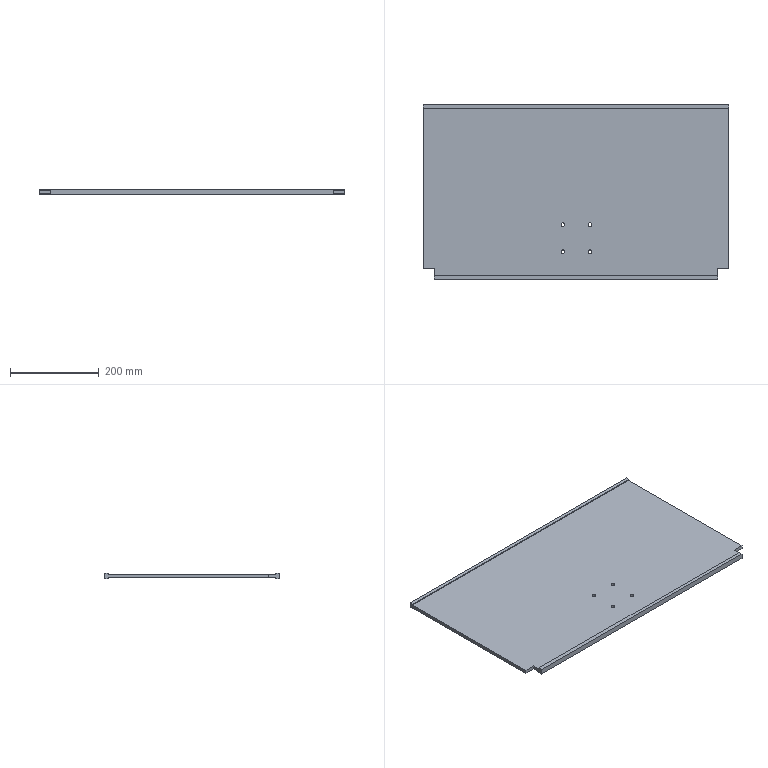Part | SolidWorks | features ICE 4, Cut 1, FlatPattern 1, SMBaseFlange 1, SheetMetal 1 | 1 solid | 26 faces | box 689 x 395 x 12 mm | volume 2213440 mm3 | plane 18 | cylinder 8 | commonest cylinder face diameters 8 x8
STEP:
#1=CARTESIAN_POINT('',(83.087,-77.137,0.));
#2=VERTEX_POINT('',#1);
#3=CARTESIAN_POINT('',(75.087,-77.137,0.));
#4=VERTEX_POINT('',#3);
#5=CARTESIAN_POINT('',(79.087,-77.137,0.));
#6=DIRECTION('',(0.,0.,-1.));
#7=DIRECTION('',(-1.,0.,0.));
#8=AXIS2_PLACEMENT_3D('',#5,#6,#7);
#9=CIRCLE('',#8,4.);
#10=EDGE_CURVE('',#2,#4,#9,.T.);
#11=ORIENTED_EDGE('',*,*,#10,.F.);
#12=CARTESIAN_POINT('',(83.087,-77.137,-8.));
#13=VERTEX_POINT('',#12);
#14=CARTESIAN_POINT('',(83.087,-77.137,2.));
#15=DIRECTION('',(0.,0.,-1.));
#16=VECTOR('',#15,1000.);
#17=LINE('',#14,#16);
#18=EDGE_CURVE('',#2,#13,#17,.T.);
#19=ORIENTED_EDGE('',*,*,#18,.T.);
#20=CARTESIAN_POINT('',(75.087,-77.137,-8.));
#21=VERTEX_POINT('',#20);
#22=CARTESIAN_POINT('',(79.087,-77.137,-8.));
#23=DIRECTION('',(0.,0.,-1.));
#24=DIRECTION('',(-1.,0.,0.));
#25=AXIS2_PLACEMENT_3D('',#22,#23,#24);
#26=CIRCLE('',#25,4.);
#27=EDGE_CURVE('',#13,#21,#26,.T.);
#28=ORIENTED_EDGE('',*,*,#27,.T.);
#29=CARTESIAN_POINT('',(75.087,-77.137,2.));
#30=DIRECTION('',(0.,0.,-1.));
#31=VECTOR('',#30,1000.);
#32=LINE('',#29,#31);
#33=EDGE_CURVE('',#4,#21,#32,.T.);
#34=ORIENTED_EDGE('',*,*,#33,.F.);
#35=EDGE_LOOP('',(#11,#19,#28,#34));
#36=FACE_OUTER_BOUND('',#35,.T.);
#37=CARTESIAN_POINT('',(79.087,-77.137,2.));
#38=DIRECTION('',(0.,0.,-1.));
#39=DIRECTION('',(-1.,0.,0.));
#40=AXIS2_PLACEMENT_3D('',#37,#38,#39);
#41=CYLINDRICAL_SURFACE('',#40,4.);
#42=ADVANCED_FACE('',(#36),#41,.F.);
#43=CARTESIAN_POINT('',(22.087,-138.137,0.));
#44=VERTEX_POINT('',#43);
#45=CARTESIAN_POINT('',(14.087,-138.137,0.));
#46=VERTEX_POINT('',#45);
#47=CARTESIAN_POINT('',(18.087,-138.137,0.));
#48=DIRECTION('',(0.,0.,-1.));
#49=DIRECTION('',(-1.,0.,0.));
#50=AXIS2_PLACEMENT_3D('',#47,#48,#49);
#51=CIRCLE('',#50,4.);
#52=EDGE_CURVE('',#44,#46,#51,.T.);
#53=ORIENTED_EDGE('',*,*,#52,.F.);
#54=CARTESIAN_POINT('',(22.087,-138.137,-8.));
#55=VERTEX_POINT('',#54);
#56=CARTESIAN_POINT('',(22.087,-138.137,2.));
#57=DIRECTION('',(0.,0.,-1.));
#58=VECTOR('',#57,1000.);
#59=LINE('',#56,#58);
#60=EDGE_CURVE('',#44,#55,#59,.T.);
#61=ORIENTED_EDGE('',*,*,#60,.T.);
#62=CARTESIAN_POINT('',(14.087,-138.137,-8.));
#63=VERTEX_POINT('',#62);
#64=CARTESIAN_POINT('',(18.087,-138.137,-8.));
#65=DIRECTION('',(0.,0.,-1.));
#66=DIRECTION('',(-1.,0.,0.));
#67=AXIS2_PLACEMENT_3D('',#64,#65,#66);
#68=CIRCLE('',#67,4.);
#69=EDGE_CURVE('',#55,#63,#68,.T.);
#70=ORIENTED_EDGE('',*,*,#69,.T.);
#71=CARTESIAN_POINT('',(14.087,-138.137,2.));
#72=DIRECTION('',(0.,0.,-1.));
#73=VECTOR('',#72,1000.);
#74=LINE('',#71,#73);
#75=EDGE_CURVE('',#46,#63,#74,.T.);
#76=ORIENTED_EDGE('',*,*,#75,.F.);
#77=EDGE_LOOP('',(#53,#61,#70,#76));
#78=FACE_OUTER_BOUND('',#77,.T.);
#79=CARTESIAN_POINT('',(18.087,-138.137,2.));
#80=DIRECTION('',(0.,0.,-1.));
#81=DIRECTION('',(-1.,0.,0.));
#82=AXIS2_PLACEMENT_3D('',#79,#80,#81);
#83=CYLINDRICAL_SURFACE('',#82,4.);
#84=ADVANCED_FACE('',(#78),#83,.F.);
#85=CARTESIAN_POINT('',(83.087,-138.137,0.));
#86=VERTEX_POINT('',#85);
#87=CARTESIAN_POINT('',(75.087,-138.137,0.));
#88=VERTEX_POINT('',#87);
#89=CARTESIAN_POINT('',(79.087,-138.137,0.));
#90=DIRECTION('',(0.,0.,-1.));
#91=DIRECTION('',(-1.,0.,0.));
#92=AXIS2_PLACEMENT_3D('',#89,#90,#91);
#93=CIRCLE('',#92,4.);
#94=EDGE_CURVE('',#86,#88,#93,.T.);
#95=ORIENTED_EDGE('',*,*,#94,.F.);
#96=CARTESIAN_POINT('',(83.087,-138.137,-8.));
#97=VERTEX_POINT('',#96);
#98=CARTESIAN_POINT('',(83.087,-138.137,2.));
#99=DIRECTION('',(0.,0.,-1.));
#100=VECTOR('',#99,1000.);
#101=LINE('',#98,#100);
#102=EDGE_CURVE('',#86,#97,#101,.T.);
#103=ORIENTED_EDGE('',*,*,#102,.T.);
#104=CARTESIAN_POINT('',(75.087,-138.137,-8.));
#105=VERTEX_POINT('',#104);
#106=CARTESIAN_POINT('',(79.087,-138.137,-8.));
#107=DIRECTION('',(0.,0.,-1.));
#108=DIRECTION('',(-1.,0.,0.));
#109=AXIS2_PLACEMENT_3D('',#106,#107,#108);
#110=CIRCLE('',#109,4.);
#111=EDGE_CURVE('',#97,#105,#110,.T.);
#112=ORIENTED_EDGE('',*,*,#111,.T.);
#113=CARTESIAN_POINT('',(75.087,-138.137,2.));
#114=DIRECTION('',(0.,0.,-1.));
#115=VECTOR('',#114,1000.);
#116=LINE('',#113,#115);
#117=EDGE_CURVE('',#88,#105,#116,.T.);
#118=ORIENTED_EDGE('',*,*,#117,.F.);
#119=EDGE_LOOP('',(#95,#103,#112,#118));
#120=FACE_OUTER_BOUND('',#119,.T.);
#121=CARTESIAN_POINT('',(79.087,-138.137,2.));
#122=DIRECTION('',(0.,0.,-1.));
#123=DIRECTION('',(-1.,0.,0.));
#124=AXIS2_PLACEMENT_3D('',#121,#122,#123);
#125=CYLINDRICAL_SURFACE('',#124,4.);
#126=ADVANCED_FACE('',(#120),#125,.F.);
#127=CARTESIAN_POINT('',(22.087,-77.137,0.));
#128=VERTEX_POINT('',#127);
#129=CARTESIAN_POINT('',(14.087,-77.137,0.));
#130=VERTEX_POINT('',#129);
#131=CARTESIAN_POINT('',(18.087,-77.137,0.));
#132=DIRECTION('',(0.,0.,-1.));
#133=DIRECTION('',(-1.,0.,0.));
#134=AXIS2_PLACEMENT_3D('',#131,#132,#133);
#135=CIRCLE('',#134,4.);
#136=EDGE_CURVE('',#128,#130,#135,.T.);
#137=ORIENTED_EDGE('',*,*,#136,.F.);
#138=CARTESIAN_POINT('',(22.087,-77.137,-8.));
#139=VERTEX_POINT('',#138);
#140=CARTESIAN_POINT('',(22.087,-77.137,2.));
#141=DIRECTION('',(0.,0.,-1.));
#142=VECTOR('',#141,1000.);
#143=LINE('',#140,#142);
#144=EDGE_CURVE('',#128,#139,#143,.T.);
#145=ORIENTED_EDGE('',*,*,#144,.T.);
#146=CARTESIAN_POINT('',(14.087,-77.137,-8.));
#147=VERTEX_POINT('',#146);
#148=CARTESIAN_POINT('',(18.087,-77.137,-8.));
#149=DIRECTION('',(0.,0.,-1.));
#150=DIRECTION('',(-1.,0.,0.));
#151=AXIS2_PLACEMENT_3D('',#148,#149,#150);
#152=CIRCLE('',#151,4.);
#153=EDGE_CURVE('',#139,#147,#152,.T.);
#154=ORIENTED_EDGE('',*,*,#153,.T.);
#155=CARTESIAN_POINT('',(14.087,-77.137,2.));
#156=DIRECTION('',(0.,0.,-1.));
#157=VECTOR('',#156,1000.);
#158=LINE('',#155,#157);
#159=EDGE_CURVE('',#130,#147,#158,.T.);
#160=ORIENTED_EDGE('',*,*,#159,.F.);
#161=EDGE_LOOP('',(#137,#145,#154,#160));
#162=FACE_OUTER_BOUND('',#161,.T.);
#163=CARTESIAN_POINT('',(18.087,-77.137,2.));
#164=DIRECTION('',(0.,0.,-1.));
#165=DIRECTION('',(-1.,0.,0.));
#166=AXIS2_PLACEMENT_3D('',#163,#164,#165);
#167=CYLINDRICAL_SURFACE('',#166,4.);
#168=ADVANCED_FACE('',(#162),#167,.F.);
#169=CARTESIAN_POINT('',(-297.,194.,-10.));
#170=VERTEX_POINT('',#169);
#171=CARTESIAN_POINT('',(-297.,194.,2.));
#172=VERTEX_POINT('',#171);
#173=CARTESIAN_POINT('',(-297.,194.,-8.));
#174=DIRECTION('',(0.,0.,1.));
#175=VECTOR('',#174,1000.);
#176=LINE('',#173,#175);
#177=EDGE_CURVE('',#170,#172,#176,.T.);
#178=ORIENTED_EDGE('',*,*,#177,.T.);
#179=CARTESIAN_POINT('',(392.,194.,2.));
#180=VERTEX_POINT('',#179);
#181=CARTESIAN_POINT('',(378.,194.,2.));
#182=DIRECTION('',(-1.,0.,0.));
#183=VECTOR('',#182,1000.);
#184=LINE('',#181,#183);
#185=EDGE_CURVE('',#180,#172,#184,.T.);
#186=ORIENTED_EDGE('',*,*,#185,.F.);
#187=CARTESIAN_POINT('',(392.,194.,-10.));
#188=VERTEX_POINT('',#187);
#189=CARTESIAN_POINT('',(392.,194.,-10.));
#190=DIRECTION('',(0.,0.,1.));
#191=VECTOR('',#190,1000.);
#192=LINE('',#189,#191);
#193=EDGE_CURVE('',#188,#180,#192,.T.);
#194=ORIENTED_EDGE('',*,*,#193,.F.);
#195=CARTESIAN_POINT('',(378.,194.,-10.));
#196=DIRECTION('',(-1.,0.,0.));
#197=VECTOR('',#196,1000.);
#198=LINE('',#195,#197);
#199=EDGE_CURVE('',#188,#170,#198,.T.);
#200=ORIENTED_EDGE('',*,*,#199,.T.);
#201=EDGE_LOOP('',(#178,#186,#194,#200));
#202=FACE_OUTER_BOUND('',#201,.T.);
#203=CARTESIAN_POINT('',(-297.,194.,-8.));
#204=DIRECTION('',(0.,1.,0.));
#205=DIRECTION('',(0.,0.,1.));
#206=AXIS2_PLACEMENT_3D('',#203,#204,#205);
#207=PLANE('',#206);
#208=ADVANCED_FACE('',(#202),#207,.T.);
#209=CARTESIAN_POINT('',(367.,-201.,-10.));
#210=VERTEX_POINT('',#209);
#211=CARTESIAN_POINT('',(367.,-201.,2.));
#212=VERTEX_POINT('',#211);
#213=CARTESIAN_POINT('',(367.,-201.,-10.));
#214=DIRECTION('',(0.,0.,1.));
#215=VECTOR('',#214,1000.);
#216=LINE('',#213,#215);
#217=EDGE_CURVE('',#210,#212,#216,.T.);
#218=ORIENTED_EDGE('',*,*,#217,.T.);
#219=CARTESIAN_POINT('',(-272.,-201.,2.));
#220=VERTEX_POINT('',#219);
#221=CARTESIAN_POINT('',(378.,-201.,2.));
#222=DIRECTION('',(-1.,0.,0.));
#223=VECTOR('',#222,1000.);
#224=LINE('',#221,#223);
#225=EDGE_CURVE('',#212,#220,#224,.T.);
#226=ORIENTED_EDGE('',*,*,#225,.T.);
#227=CARTESIAN_POINT('',(-272.,-201.,-10.));
#228=VERTEX_POINT('',#227);
#229=CARTESIAN_POINT('',(-272.,-201.,-10.));
#230=DIRECTION('',(0.,0.,1.));
#231=VECTOR('',#230,1000.);
#232=LINE('',#229,#231);
#233=EDGE_CURVE('',#228,#220,#232,.T.);
#234=ORIENTED_EDGE('',*,*,#233,.F.);
#235=CARTESIAN_POINT('',(378.,-201.,-10.));
#236=DIRECTION('',(-1.,0.,0.));
#237=VECTOR('',#236,1000.);
#238=LINE('',#235,#237);
#239=EDGE_CURVE('',#210,#228,#238,.T.);
#240=ORIENTED_EDGE('',*,*,#239,.F.);
#241=EDGE_LOOP('',(#218,#226,#234,#240));
#242=FACE_OUTER_BOUND('',#241,.T.);
#243=CARTESIAN_POINT('',(-297.,-201.,-8.));
#244=DIRECTION('',(0.,-1.,0.));
#245=DIRECTION('',(0.,0.,-1.));
#246=AXIS2_PLACEMENT_3D('',#243,#244,#245);
#247=PLANE('',#246);
#248=ADVANCED_FACE('',(#242),#247,.T.);
#249=CARTESIAN_POINT('',(-297.,-176.,-8.));
#250=VERTEX_POINT('',#249);
#251=CARTESIAN_POINT('',(-297.,-176.,0.));
#252=VERTEX_POINT('',#251);
#253=CARTESIAN_POINT('',(-297.,-176.,-10.));
#254=DIRECTION('',(0.,0.,1.));
#255=VECTOR('',#254,1000.);
#256=LINE('',#253,#255);
#257=EDGE_CURVE('',#250,#252,#256,.T.);
#258=ORIENTED_EDGE('',*,*,#257,.T.);
#259=CARTESIAN_POINT('',(-297.,185.,0.));
#260=VERTEX_POINT('',#259);
#261=CARTESIAN_POINT('',(-297.,194.,0.));
#262=DIRECTION('',(0.,-1.,0.));
#263=VECTOR('',#262,1000.);
#264=LINE('',#261,#263);
#265=EDGE_CURVE('',#260,#252,#264,.T.);
#266=ORIENTED_EDGE('',*,*,#265,.F.);
#267=CARTESIAN_POINT('',(-297.,185.,2.));
#268=VERTEX_POINT('',#267);
#269=CARTESIAN_POINT('',(-297.,185.,-10.));
#270=DIRECTION('',(0.,0.,1.));
#271=VECTOR('',#270,1000.);
#272=LINE('',#269,#271);
#273=EDGE_CURVE('',#260,#268,#272,.T.);
#274=ORIENTED_EDGE('',*,*,#273,.T.);
#275=CARTESIAN_POINT('',(-297.,194.,2.));
#276=DIRECTION('',(0.,1.,0.));
#277=VECTOR('',#276,1000.);
#278=LINE('',#275,#277);
#279=EDGE_CURVE('',#268,#172,#278,.T.);
#280=ORIENTED_EDGE('',*,*,#279,.T.);
#281=ORIENTED_EDGE('',*,*,#177,.F.);
#282=CARTESIAN_POINT('',(-297.,185.,-10.));
#283=VERTEX_POINT('',#282);
#284=CARTESIAN_POINT('',(-297.,194.,-10.));
#285=DIRECTION('',(0.,-1.,0.));
#286=VECTOR('',#285,1000.);
#287=LINE('',#284,#286);
#288=EDGE_CURVE('',#170,#283,#287,.T.);
#289=ORIENTED_EDGE('',*,*,#288,.T.);
#290=CARTESIAN_POINT('',(-297.,185.,-8.));
#291=VERTEX_POINT('',#290);
#292=CARTESIAN_POINT('',(-297.,185.,-10.));
#293=DIRECTION('',(0.,0.,1.));
#294=VECTOR('',#293,1000.);
#295=LINE('',#292,#294);
#296=EDGE_CURVE('',#283,#291,#295,.T.);
#297=ORIENTED_EDGE('',*,*,#296,.T.);
#298=CARTESIAN_POINT('',(-297.,194.,-8.));
#299=DIRECTION('',(0.,-1.,0.));
#300=VECTOR('',#299,1000.);
#301=LINE('',#298,#300);
#302=EDGE_CURVE('',#291,#250,#301,.T.);
#303=ORIENTED_EDGE('',*,*,#302,.T.);
#304=EDGE_LOOP('',(#258,#266,#274,#280,#281,#289,#297,#303));
#305=FACE_OUTER_BOUND('',#304,.T.);
#306=CARTESIAN_POINT('',(-297.,194.,-8.));
#307=DIRECTION('',(-1.,0.,0.));
#308=DIRECTION('',(0.,0.,1.));
#309=AXIS2_PLACEMENT_3D('',#306,#307,#308);
#310=PLANE('',#309);
#311=ADVANCED_FACE('',(#305),#310,.T.);
#312=CARTESIAN_POINT('',(367.,-192.,-8.));
#313=VERTEX_POINT('',#312);
#314=CARTESIAN_POINT('',(367.,-176.,-8.));
#315=VERTEX_POINT('',#314);
#316=CARTESIAN_POINT('',(367.,0.,-8.));
#317=DIRECTION('',(0.,1.,0.));
#318=VECTOR('',#317,1000.);
#319=LINE('',#316,#318);
#320=EDGE_CURVE('',#313,#315,#319,.T.);
#321=ORIENTED_EDGE('',*,*,#320,.F.);
#322=CARTESIAN_POINT('',(-272.,-192.,-8.));
#323=VERTEX_POINT('',#322);
#324=CARTESIAN_POINT('',(0.,-192.,-8.));
#325=DIRECTION('',(1.,0.,0.));
#326=VECTOR('',#325,1000.);
#327=LINE('',#324,#326);
#328=EDGE_CURVE('',#323,#313,#327,.T.);
#329=ORIENTED_EDGE('',*,*,#328,.F.);
#330=CARTESIAN_POINT('',(-272.,-176.,-8.));
#331=VERTEX_POINT('',#330);
#332=CARTESIAN_POINT('',(-272.,0.,-8.));
#333=DIRECTION('',(0.,-1.,0.));
#334=VECTOR('',#333,1000.);
#335=LINE('',#332,#334);
#336=EDGE_CURVE('',#331,#323,#335,.T.);
#337=ORIENTED_EDGE('',*,*,#336,.F.);
#338=CARTESIAN_POINT('',(0.,-176.,-8.));
#339=DIRECTION('',(1.,0.,0.));
#340=VECTOR('',#339,1000.);
#341=LINE('',#338,#340);
#342=EDGE_CURVE('',#250,#331,#341,.T.);
#343=ORIENTED_EDGE('',*,*,#342,.F.);
#344=ORIENTED_EDGE('',*,*,#302,.F.);
#345=CARTESIAN_POINT('',(392.,185.,-8.));
#346=VERTEX_POINT('',#345);
#347=CARTESIAN_POINT('',(0.,185.,-8.));
#348=DIRECTION('',(-1.,0.,0.));
#349=VECTOR('',#348,1000.);
#350=LINE('',#347,#349);
#351=EDGE_CURVE('',#346,#291,#350,.T.);
#352=ORIENTED_EDGE('',*,*,#351,.F.);
#353=CARTESIAN_POINT('',(392.,-176.,-8.));
#354=VERTEX_POINT('',#353);
#355=CARTESIAN_POINT('',(392.,-192.,-8.));
#356=DIRECTION('',(0.,1.,0.));
#357=VECTOR('',#356,1000.);
#358=LINE('',#355,#357);
#359=EDGE_CURVE('',#354,#346,#358,.T.);
#360=ORIENTED_EDGE('',*,*,#359,.F.);
#361=CARTESIAN_POINT('',(0.,-176.,-8.));
#362=DIRECTION('',(1.,0.,0.));
#363=VECTOR('',#362,1000.);
#364=LINE('',#361,#363);
#365=EDGE_CURVE('',#315,#354,#364,.T.);
#366=ORIENTED_EDGE('',*,*,#365,.F.);
#367=EDGE_LOOP('',(#321,#329,#337,#343,#344,#352,#360,#366));
#368=FACE_OUTER_BOUND('',#367,.T.);
#369=CARTESIAN_POINT('',(79.087,-77.137,-8.));
#370=DIRECTION('',(0.,0.,-1.));
#371=DIRECTION('',(-1.,0.,0.));
#372=AXIS2_PLACEMENT_3D('',#369,#370,#371);
#373=CIRCLE('',#372,4.);
#374=EDGE_CURVE('',#21,#13,#373,.T.);
#375=ORIENTED_EDGE('',*,*,#374,.F.);
#376=ORIENTED_EDGE('',*,*,#27,.F.);
#377=EDGE_LOOP('',(#375,#376));
#378=FACE_BOUND('',#377,.T.);
#379=CARTESIAN_POINT('',(18.087,-138.137,-8.));
#380=DIRECTION('',(0.,0.,-1.));
#381=DIRECTION('',(-1.,0.,0.));
#382=AXIS2_PLACEMENT_3D('',#379,#380,#381);
#383=CIRCLE('',#382,4.);
#384=EDGE_CURVE('',#63,#55,#383,.T.);
#385=ORIENTED_EDGE('',*,*,#384,.F.);
#386=ORIENTED_EDGE('',*,*,#69,.F.);
#387=EDGE_LOOP('',(#385,#386));
#388=FACE_BOUND('',#387,.T.);
#389=CARTESIAN_POINT('',(79.087,-138.137,-8.));
#390=DIRECTION('',(0.,0.,-1.));
#391=DIRECTION('',(-1.,0.,0.));
#392=AXIS2_PLACEMENT_3D('',#389,#390,#391);
#393=CIRCLE('',#392,4.);
#394=EDGE_CURVE('',#105,#97,#393,.T.);
#395=ORIENTED_EDGE('',*,*,#394,.F.);
#396=ORIENTED_EDGE('',*,*,#111,.F.);
#397=EDGE_LOOP('',(#395,#396));
#398=FACE_BOUND('',#397,.T.);
#399=CARTESIAN_POINT('',(18.087,-77.137,-8.));
#400=DIRECTION('',(0.,0.,-1.));
#401=DIRECTION('',(-1.,0.,0.));
#402=AXIS2_PLACEMENT_3D('',#399,#400,#401);
#403=CIRCLE('',#402,4.);
#404=EDGE_CURVE('',#147,#139,#403,.T.);
#405=ORIENTED_EDGE('',*,*,#404,.F.);
#406=ORIENTED_EDGE('',*,*,#153,.F.);
#407=EDGE_LOOP('',(#405,#406));
#408=FACE_BOUND('',#407,.T.);
#409=CARTESIAN_POINT('',(0.,0.,-8.));
#410=DIRECTION('',(0.,0.,-1.));
#411=DIRECTION('',(-1.,0.,0.));
#412=AXIS2_PLACEMENT_3D('',#409,#410,#411);
#413=PLANE('',#412);
#414=ADVANCED_FACE('',(#368,#378,#388,#398,#408),#413,.T.);
#415=CARTESIAN_POINT('',(79.087,-77.137,0.));
#416=DIRECTION('',(0.,0.,-1.));
#417=DIRECTION('',(-1.,0.,0.));
#418=AXIS2_PLACEMENT_3D('',#415,#416,#417);
#419=CIRCLE('',#418,4.);
#420=EDGE_CURVE('',#4,#2,#419,.T.);
#421=ORIENTED_EDGE('',*,*,#420,.T.);
#422=ORIENTED_EDGE('',*,*,#10,.T.);
#423=EDGE_LOOP('',(#421,#422));
#424=FACE_BOUND('',#423,.T.);
#425=CARTESIAN_POINT('',(18.087,-138.137,0.));
#426=DIRECTION('',(0.,0.,-1.));
#427=DIRECTION('',(-1.,0.,0.));
#428=AXIS2_PLACEMENT_3D('',#425,#426,#427);
#429=CIRCLE('',#428,4.);
#430=EDGE_CURVE('',#46,#44,#429,.T.);
#431=ORIENTED_EDGE('',*,*,#430,.T.);
#432=ORIENTED_EDGE('',*,*,#52,.T.);
#433=EDGE_LOOP('',(#431,#432));
#434=FACE_BOUND('',#433,.T.);
#435=CARTESIAN_POINT('',(79.087,-138.137,0.));
#436=DIRECTION('',(0.,0.,-1.));
#437=DIRECTION('',(-1.,0.,0.));
#438=AXIS2_PLACEMENT_3D('',#435,#436,#437);
#439=CIRCLE('',#438,4.);
#440=EDGE_CURVE('',#88,#86,#439,.T.);
#441=ORIENTED_EDGE('',*,*,#440,.T.);
#442=ORIENTED_EDGE('',*,*,#94,.T.);
#443=EDGE_LOOP('',(#441,#442));
#444=FACE_BOUND('',#443,.T.);
#445=CARTESIAN_POINT('',(18.087,-77.137,0.));
#446=DIRECTION('',(0.,0.,-1.));
#447=DIRECTION('',(-1.,0.,0.));
#448=AXIS2_PLACEMENT_3D('',#445,#446,#447);
#449=CIRCLE('',#448,4.);
#450=EDGE_CURVE('',#130,#128,#449,.T.);
#451=ORIENTED_EDGE('',*,*,#450,.T.);
#452=ORIENTED_EDGE('',*,*,#136,.T.);
#453=EDGE_LOOP('',(#451,#452));
#454=FACE_BOUND('',#453,.T.);
#455=CARTESIAN_POINT('',(-272.,-192.,0.));
#456=VERTEX_POINT('',#455);
#457=CARTESIAN_POINT('',(367.,-192.,0.));
#458=VERTEX_POINT('',#457);
#459=CARTESIAN_POINT('',(0.,-192.,0.));
#460=DIRECTION('',(1.,0.,0.));
#461=VECTOR('',#460,1000.);
#462=LINE('',#459,#461);
#463=EDGE_CURVE('',#456,#458,#462,.T.);
#464=ORIENTED_EDGE('',*,*,#463,.T.);
#465=CARTESIAN_POINT('',(367.,-176.,0.));
#466=VERTEX_POINT('',#465);
#467=CARTESIAN_POINT('',(367.,0.,0.));
#468=DIRECTION('',(0.,1.,0.));
#469=VECTOR('',#468,1000.);
#470=LINE('',#467,#469);
#471=EDGE_CURVE('',#458,#466,#470,.T.);
#472=ORIENTED_EDGE('',*,*,#471,.T.);
#473=CARTESIAN_POINT('',(392.,-176.,0.));
#474=VERTEX_POINT('',#473);
#475=CARTESIAN_POINT('',(0.,-176.,0.));
#476=DIRECTION('',(1.,0.,0.));
#477=VECTOR('',#476,1000.);
#478=LINE('',#475,#477);
#479=EDGE_CURVE('',#466,#474,#478,.T.);
#480=ORIENTED_EDGE('',*,*,#479,.T.);
#481=CARTESIAN_POINT('',(392.,185.,0.));
#482=VERTEX_POINT('',#481);
#483=CARTESIAN_POINT('',(392.,185.,0.));
#484=DIRECTION('',(0.,-1.,0.));
#485=VECTOR('',#484,1000.);
#486=LINE('',#483,#485);
#487=EDGE_CURVE('',#482,#474,#486,.T.);
#488=ORIENTED_EDGE('',*,*,#487,.F.);
#489=CARTESIAN_POINT('',(0.,185.,0.));
#490=DIRECTION('',(-1.,0.,0.));
#491=VECTOR('',#490,1000.);
#492=LINE('',#489,#491);
#493=EDGE_CURVE('',#482,#260,#492,.T.);
#494=ORIENTED_EDGE('',*,*,#493,.T.);
#495=ORIENTED_EDGE('',*,*,#265,.T.);
#496=CARTESIAN_POINT('',(-272.,-176.,0.));
#497=VERTEX_POINT('',#496);
#498=CARTESIAN_POINT('',(0.,-176.,0.));
#499=DIRECTION('',(1.,0.,0.));
#500=VECTOR('',#499,1000.);
#501=LINE('',#498,#500);
#502=EDGE_CURVE('',#252,#497,#501,.T.);
#503=ORIENTED_EDGE('',*,*,#502,.T.);
#504=CARTESIAN_POINT('',(-272.,0.,0.));
#505=DIRECTION('',(0.,-1.,0.));
#506=VECTOR('',#505,1000.);
#507=LINE('',#504,#506);
#508=EDGE_CURVE('',#497,#456,#507,.T.);
#509=ORIENTED_EDGE('',*,*,#508,.T.);
#510=EDGE_LOOP('',(#464,#472,#480,#488,#494,#495,#503,#509));
#511=FACE_OUTER_BOUND('',#510,.T.);
#512=CARTESIAN_POINT('',(0.,0.,0.));
#513=DIRECTION('',(0.,0.,-1.));
#514=DIRECTION('',(-1.,0.,0.));
#515=AXIS2_PLACEMENT_3D('',#512,#513,#514);
#516=PLANE('',#515);
#517=ADVANCED_FACE('',(#424,#434,#444,#454,#511),#516,.F.);
#518=CARTESIAN_POINT('',(367.,-192.,2.));
#519=VERTEX_POINT('',#518);
#520=CARTESIAN_POINT('',(367.,-201.,2.));
#521=DIRECTION('',(0.,-1.,0.));
#522=VECTOR('',#521,1000.);
#523=LINE('',#520,#522);
#524=EDGE_CURVE('',#519,#212,#523,.T.);
#525=ORIENTED_EDGE('',*,*,#524,.F.);
#526=CARTESIAN_POINT('',(-272.,-192.,2.));
#527=VERTEX_POINT('',#526);
#528=CARTESIAN_POINT('',(378.,-192.,2.));
#529=DIRECTION('',(-1.,0.,0.));
#530=VECTOR('',#529,1000.);
#531=LINE('',#528,#530);
#532=EDGE_CURVE('',#519,#527,#531,.T.);
#533=ORIENTED_EDGE('',*,*,#532,.T.);
#534=CARTESIAN_POINT('',(-272.,-201.,2.));
#535=DIRECTION('',(0.,1.,0.));
#536=VECTOR('',#535,1000.);
#537=LINE('',#534,#536);
#538=EDGE_CURVE('',#220,#527,#537,.T.);
#539=ORIENTED_EDGE('',*,*,#538,.F.);
#540=ORIENTED_EDGE('',*,*,#225,.F.);
#541=EDGE_LOOP('',(#525,#533,#539,#540));
#542=FACE_OUTER_BOUND('',#541,.T.);
#543=CARTESIAN_POINT('',(378.,-201.,2.));
#544=DIRECTION('',(0.,0.,1.));
#545=DIRECTION('',(1.,0.,0.));
#546=AXIS2_PLACEMENT_3D('',#543,#544,#545);
#547=PLANE('',#546);
#548=ADVANCED_FACE('',(#542),#547,.T.);
#549=CARTESIAN_POINT('',(367.,-192.,-10.));
#550=DIRECTION('',(0.,0.,1.));
#551=VECTOR('',#550,1000.);
#552=LINE('',#549,#551);
#553=EDGE_CURVE('',#458,#519,#552,.T.);
#554=ORIENTED_EDGE('',*,*,#553,.F.);
#555=ORIENTED_EDGE('',*,*,#463,.F.);
#556=CARTESIAN_POINT('',(-272.,-192.,-10.));
#557=DIRECTION('',(0.,0.,-1.));
#558=VECTOR('',#557,1000.);
#559=LINE('',#556,#558);
#560=EDGE_CURVE('',#527,#456,#559,.T.);
#561=ORIENTED_EDGE('',*,*,#560,.F.);
#562=ORIENTED_EDGE('',*,*,#532,.F.);
#563=EDGE_LOOP('',(#554,#555,#561,#562));
#564=FACE_OUTER_BOUND('',#563,.T.);
#565=CARTESIAN_POINT('',(378.,-192.,-10.));
#566=DIRECTION('',(0.,1.,0.));
#567=DIRECTION('',(0.,0.,1.));
#568=AXIS2_PLACEMENT_3D('',#565,#566,#567);
#569=PLANE('',#568);
#570=ADVANCED_FACE('',(#564),#569,.T.);
#571=CARTESIAN_POINT('',(367.,-192.,-10.));
#572=VERTEX_POINT('',#571);
#573=CARTESIAN_POINT('',(367.,-192.,-10.));
#574=DIRECTION('',(0.,0.,1.));
#575=VECTOR('',#574,1000.);
#576=LINE('',#573,#575);
#577=EDGE_CURVE('',#572,#313,#576,.T.);
#578=ORIENTED_EDGE('',*,*,#577,.F.);
#579=CARTESIAN_POINT('',(-272.,-192.,-10.));
#580=VERTEX_POINT('',#579);
#581=CARTESIAN_POINT('',(378.,-192.,-10.));
#582=DIRECTION('',(-1.,0.,0.));
#583=VECTOR('',#582,1000.);
#584=LINE('',#581,#583);
#585=EDGE_CURVE('',#572,#580,#584,.T.);
#586=ORIENTED_EDGE('',*,*,#585,.T.);
#587=CARTESIAN_POINT('',(-272.,-192.,-10.));
#588=DIRECTION('',(0.,0.,-1.));
#589=VECTOR('',#588,1000.);
#590=LINE('',#587,#589);
#591=EDGE_CURVE('',#323,#580,#590,.T.);
#592=ORIENTED_EDGE('',*,*,#591,.F.);
#593=ORIENTED_EDGE('',*,*,#328,.T.);
#594=EDGE_LOOP('',(#578,#586,#592,#593));
#595=FACE_OUTER_BOUND('',#594,.T.);
#596=CARTESIAN_POINT('',(378.,-192.,-10.));
#597=DIRECTION('',(0.,1.,0.));
#598=DIRECTION('',(0.,0.,1.));
#599=AXIS2_PLACEMENT_3D('',#596,#597,#598);
#600=PLANE('',#599);
#601=ADVANCED_FACE('',(#595),#600,.T.);
#602=CARTESIAN_POINT('',(367.,-201.,-10.));
#603=DIRECTION('',(0.,-1.,0.));
#604=VECTOR('',#603,1000.);
#605=LINE('',#602,#604);
#606=EDGE_CURVE('',#572,#210,#605,.T.);
#607=ORIENTED_EDGE('',*,*,#606,.T.);
#608=ORIENTED_EDGE('',*,*,#239,.T.);
#609=CARTESIAN_POINT('',(-272.,-201.,-10.));
#610=DIRECTION('',(0.,1.,0.));
#611=VECTOR('',#610,1000.);
#612=LINE('',#609,#611);
#613=EDGE_CURVE('',#228,#580,#612,.T.);
#614=ORIENTED_EDGE('',*,*,#613,.T.);
#615=ORIENTED_EDGE('',*,*,#585,.F.);
#616=EDGE_LOOP('',(#607,#608,#614,#615));
#617=FACE_OUTER_BOUND('',#616,.T.);
#618=CARTESIAN_POINT('',(378.,-201.,-10.));
#619=DIRECTION('',(0.,0.,-1.));
#620=DIRECTION('',(-1.,0.,0.));
#621=AXIS2_PLACEMENT_3D('',#618,#619,#620);
#622=PLANE('',#621);
#623=ADVANCED_FACE('',(#617),#622,.T.);
#624=CARTESIAN_POINT('',(392.,185.,2.));
#625=VERTEX_POINT('',#624);
#626=CARTESIAN_POINT('',(378.,185.,2.));
#627=DIRECTION('',(-1.,0.,0.));
#628=VECTOR('',#627,1000.);
#629=LINE('',#626,#628);
#630=EDGE_CURVE('',#625,#268,#629,.T.);
#631=ORIENTED_EDGE('',*,*,#630,.F.);
#632=CARTESIAN_POINT('',(392.,194.,2.));
#633=DIRECTION('',(0.,-1.,0.));
#634=VECTOR('',#633,1000.);
#635=LINE('',#632,#634);
#636=EDGE_CURVE('',#180,#625,#635,.T.);
#637=ORIENTED_EDGE('',*,*,#636,.F.);
#638=ORIENTED_EDGE('',*,*,#185,.T.);
#639=ORIENTED_EDGE('',*,*,#279,.F.);
#640=EDGE_LOOP('',(#631,#637,#638,#639));
#641=FACE_OUTER_BOUND('',#640,.T.);
#642=CARTESIAN_POINT('',(378.,194.,2.));
#643=DIRECTION('',(0.,0.,1.));
#644=DIRECTION('',(1.,0.,0.));
#645=AXIS2_PLACEMENT_3D('',#642,#643,#644);
#646=PLANE('',#645);
#647=ADVANCED_FACE('',(#641),#646,.T.);
#648=ORIENTED_EDGE('',*,*,#493,.F.);
#649=CARTESIAN_POINT('',(392.,185.,2.));
#650=DIRECTION('',(0.,0.,-1.));
#651=VECTOR('',#650,1000.);
#652=LINE('',#649,#651);
#653=EDGE_CURVE('',#625,#482,#652,.T.);
#654=ORIENTED_EDGE('',*,*,#653,.F.);
#655=ORIENTED_EDGE('',*,*,#630,.T.);
#656=ORIENTED_EDGE('',*,*,#273,.F.);
#657=EDGE_LOOP('',(#648,#654,#655,#656));
#658=FACE_OUTER_BOUND('',#657,.T.);
#659=CARTESIAN_POINT('',(378.,185.,-10.));
#660=DIRECTION('',(0.,-1.,0.));
#661=DIRECTION('',(0.,0.,-1.));
#662=AXIS2_PLACEMENT_3D('',#659,#660,#661);
#663=PLANE('',#662);
#664=ADVANCED_FACE('',(#658),#663,.T.);
#665=ORIENTED_EDGE('',*,*,#199,.F.);
#666=CARTESIAN_POINT('',(392.,185.,-10.));
#667=VERTEX_POINT('',#666);
#668=CARTESIAN_POINT('',(392.,185.,-10.));
#669=DIRECTION('',(0.,1.,0.));
#670=VECTOR('',#669,1000.);
#671=LINE('',#668,#670);
#672=EDGE_CURVE('',#667,#188,#671,.T.);
#673=ORIENTED_EDGE('',*,*,#672,.F.);
#674=CARTESIAN_POINT('',(378.,185.,-10.));
#675=DIRECTION('',(-1.,0.,0.));
#676=VECTOR('',#675,1000.);
#677=LINE('',#674,#676);
#678=EDGE_CURVE('',#667,#283,#677,.T.);
#679=ORIENTED_EDGE('',*,*,#678,.T.);
#680=ORIENTED_EDGE('',*,*,#288,.F.);
#681=EDGE_LOOP('',(#665,#673,#679,#680));
#682=FACE_OUTER_BOUND('',#681,.T.);
#683=CARTESIAN_POINT('',(378.,194.,-10.));
#684=DIRECTION('',(0.,0.,-1.));
#685=DIRECTION('',(-1.,0.,0.));
#686=AXIS2_PLACEMENT_3D('',#683,#684,#685);
#687=PLANE('',#686);
#688=ADVANCED_FACE('',(#682),#687,.T.);
#689=ORIENTED_EDGE('',*,*,#678,.F.);
#690=CARTESIAN_POINT('',(392.,185.,-8.));
#691=DIRECTION('',(0.,0.,-1.));
#692=VECTOR('',#691,1000.);
#693=LINE('',#690,#692);
#694=EDGE_CURVE('',#346,#667,#693,.T.);
#695=ORIENTED_EDGE('',*,*,#694,.F.);
#696=ORIENTED_EDGE('',*,*,#351,.T.);
#697=ORIENTED_EDGE('',*,*,#296,.F.);
#698=EDGE_LOOP('',(#689,#695,#696,#697));
#699=FACE_OUTER_BOUND('',#698,.T.);
#700=CARTESIAN_POINT('',(378.,185.,-10.));
#701=DIRECTION('',(0.,-1.,0.));
#702=DIRECTION('',(0.,0.,-1.));
#703=AXIS2_PLACEMENT_3D('',#700,#701,#702);
#704=PLANE('',#703);
#705=ADVANCED_FACE('',(#699),#704,.T.);
#706=ORIENTED_EDGE('',*,*,#144,.F.);
#707=ORIENTED_EDGE('',*,*,#450,.F.);
#708=ORIENTED_EDGE('',*,*,#159,.T.);
#709=ORIENTED_EDGE('',*,*,#404,.T.);
#710=EDGE_LOOP('',(#706,#707,#708,#709));
#711=FACE_OUTER_BOUND('',#710,.T.);
#712=CARTESIAN_POINT('',(18.087,-77.137,2.));
#713=DIRECTION('',(0.,0.,-1.));
#714=DIRECTION('',(-1.,0.,0.));
#715=AXIS2_PLACEMENT_3D('',#712,#713,#714);
#716=CYLINDRICAL_SURFACE('',#715,4.);
#717=ADVANCED_FACE('',(#711),#716,.F.);
#718=ORIENTED_EDGE('',*,*,#102,.F.);
#719=ORIENTED_EDGE('',*,*,#440,.F.);
#720=ORIENTED_EDGE('',*,*,#117,.T.);
#721=ORIENTED_EDGE('',*,*,#394,.T.);
#722=EDGE_LOOP('',(#718,#719,#720,#721));
#723=FACE_OUTER_BOUND('',#722,.T.);
#724=CARTESIAN_POINT('',(79.087,-138.137,2.));
#725=DIRECTION('',(0.,0.,-1.));
#726=DIRECTION('',(-1.,0.,0.));
#727=AXIS2_PLACEMENT_3D('',#724,#725,#726);
#728=CYLINDRICAL_SURFACE('',#727,4.);
#729=ADVANCED_FACE('',(#723),#728,.F.);
#730=ORIENTED_EDGE('',*,*,#60,.F.);
#731=ORIENTED_EDGE('',*,*,#430,.F.);
#732=ORIENTED_EDGE('',*,*,#75,.T.);
#733=ORIENTED_EDGE('',*,*,#384,.T.);
#734=EDGE_LOOP('',(#730,#731,#732,#733));
#735=FACE_OUTER_BOUND('',#734,.T.);
#736=CARTESIAN_POINT('',(18.087,-138.137,2.));
#737=DIRECTION('',(0.,0.,-1.));
#738=DIRECTION('',(-1.,0.,0.));
#739=AXIS2_PLACEMENT_3D('',#736,#737,#738);
#740=CYLINDRICAL_SURFACE('',#739,4.);
#741=ADVANCED_FACE('',(#735),#740,.F.);
#742=ORIENTED_EDGE('',*,*,#18,.F.);
#743=ORIENTED_EDGE('',*,*,#420,.F.);
#744=ORIENTED_EDGE('',*,*,#33,.T.);
#745=ORIENTED_EDGE('',*,*,#374,.T.);
#746=EDGE_LOOP('',(#742,#743,#744,#745));
#747=FACE_OUTER_BOUND('',#746,.T.);
#748=CARTESIAN_POINT('',(79.087,-77.137,2.));
#749=DIRECTION('',(0.,0.,-1.));
#750=DIRECTION('',(-1.,0.,0.));
#751=AXIS2_PLACEMENT_3D('',#748,#749,#750);
#752=CYLINDRICAL_SURFACE('',#751,4.);
#753=ADVANCED_FACE('',(#747),#752,.F.);
#754=ORIENTED_EDGE('',*,*,#342,.T.);
#755=CARTESIAN_POINT('',(-272.,-176.,-10.));
#756=DIRECTION('',(0.,0.,1.));
#757=VECTOR('',#756,1000.);
#758=LINE('',#755,#757);
#759=EDGE_CURVE('',#331,#497,#758,.T.);
#760=ORIENTED_EDGE('',*,*,#759,.T.);
#761=ORIENTED_EDGE('',*,*,#502,.F.);
#762=ORIENTED_EDGE('',*,*,#257,.F.);
#763=EDGE_LOOP('',(#754,#760,#761,#762));
#764=FACE_OUTER_BOUND('',#763,.T.);
#765=CARTESIAN_POINT('',(-297.,-176.,-10.));
#766=DIRECTION('',(0.,1.,0.));
#767=DIRECTION('',(0.,0.,1.));
#768=AXIS2_PLACEMENT_3D('',#765,#766,#767);
#769=PLANE('',#768);
#770=ADVANCED_FACE('',(#764),#769,.F.);
#771=ORIENTED_EDGE('',*,*,#759,.F.);
#772=ORIENTED_EDGE('',*,*,#336,.T.);
#773=ORIENTED_EDGE('',*,*,#591,.T.);
#774=ORIENTED_EDGE('',*,*,#613,.F.);
#775=ORIENTED_EDGE('',*,*,#233,.T.);
#776=ORIENTED_EDGE('',*,*,#538,.T.);
#777=ORIENTED_EDGE('',*,*,#560,.T.);
#778=ORIENTED_EDGE('',*,*,#508,.F.);
#779=EDGE_LOOP('',(#771,#772,#773,#774,#775,#776,#777,#778));
#780=FACE_OUTER_BOUND('',#779,.T.);
#781=CARTESIAN_POINT('',(-272.,-201.,-10.));
#782=DIRECTION('',(1.,0.,0.));
#783=DIRECTION('',(0.,0.,-1.));
#784=AXIS2_PLACEMENT_3D('',#781,#782,#783);
#785=PLANE('',#784);
#786=ADVANCED_FACE('',(#780),#785,.F.);
#787=ORIENTED_EDGE('',*,*,#487,.T.);
#788=CARTESIAN_POINT('',(392.,-176.,0.));
#789=DIRECTION('',(0.,0.,-1.));
#790=VECTOR('',#789,1000.);
#791=LINE('',#788,#790);
#792=EDGE_CURVE('',#474,#354,#791,.T.);
#793=ORIENTED_EDGE('',*,*,#792,.T.);
#794=ORIENTED_EDGE('',*,*,#359,.T.);
#795=ORIENTED_EDGE('',*,*,#694,.T.);
#796=ORIENTED_EDGE('',*,*,#672,.T.);
#797=ORIENTED_EDGE('',*,*,#193,.T.);
#798=ORIENTED_EDGE('',*,*,#636,.T.);
#799=ORIENTED_EDGE('',*,*,#653,.T.);
#800=EDGE_LOOP('',(#787,#793,#794,#795,#796,#797,#798,#799));
#801=FACE_OUTER_BOUND('',#800,.T.);
#802=CARTESIAN_POINT('',(392.,0.,0.));
#803=DIRECTION('',(-1.,0.,0.));
#804=DIRECTION('',(0.,0.,1.));
#805=AXIS2_PLACEMENT_3D('',#802,#803,#804);
#806=PLANE('',#805);
#807=ADVANCED_FACE('',(#801),#806,.F.);
#808=ORIENTED_EDGE('',*,*,#553,.T.);
#809=ORIENTED_EDGE('',*,*,#524,.T.);
#810=ORIENTED_EDGE('',*,*,#217,.F.);
#811=ORIENTED_EDGE('',*,*,#606,.F.);
#812=ORIENTED_EDGE('',*,*,#577,.T.);
#813=ORIENTED_EDGE('',*,*,#320,.T.);
#814=CARTESIAN_POINT('',(367.,-176.,-10.));
#815=DIRECTION('',(0.,0.,1.));
#816=VECTOR('',#815,1000.);
#817=LINE('',#814,#816);
#818=EDGE_CURVE('',#315,#466,#817,.T.);
#819=ORIENTED_EDGE('',*,*,#818,.T.);
#820=ORIENTED_EDGE('',*,*,#471,.F.);
#821=EDGE_LOOP('',(#808,#809,#810,#811,#812,#813,#819,#820));
#822=FACE_OUTER_BOUND('',#821,.T.);
#823=CARTESIAN_POINT('',(367.,-201.,-10.));
#824=DIRECTION('',(-1.,0.,0.));
#825=DIRECTION('',(0.,0.,1.));
#826=AXIS2_PLACEMENT_3D('',#823,#824,#825);
#827=PLANE('',#826);
#828=ADVANCED_FACE('',(#822),#827,.F.);
#829=ORIENTED_EDGE('',*,*,#365,.T.);
#830=ORIENTED_EDGE('',*,*,#792,.F.);
#831=ORIENTED_EDGE('',*,*,#479,.F.);
#832=ORIENTED_EDGE('',*,*,#818,.F.);
#833=EDGE_LOOP('',(#829,#830,#831,#832));
#834=FACE_OUTER_BOUND('',#833,.T.);
#835=CARTESIAN_POINT('',(392.,-176.,-10.));
#836=DIRECTION('',(0.,1.,0.));
#837=DIRECTION('',(0.,0.,1.));
#838=AXIS2_PLACEMENT_3D('',#835,#836,#837);
#839=PLANE('',#838);
#840=ADVANCED_FACE('',(#834),#839,.F.);
#841=CLOSED_SHELL('',(#42,#84,#126,#168,#208,#248,#311,#414,#517,#548,#570,#601,#623,#647,#664,#688,#705,#717,#729,#741,#753,#770,#786,#807,#828,#840));
#842=MANIFOLD_SOLID_BREP('',#841);
#843=CARTESIAN_POINT('',(0.,0.,0.));
#844=DIRECTION('',(0.,0.,1.));
#845=DIRECTION('',(1.,0.,0.));
#846=AXIS2_PLACEMENT_3D('',#843,#844,#845);
#847=(LENGTH_UNIT()NAMED_UNIT(*)SI_UNIT(.MILLI.,.METRE.));
#848=UNCERTAINTY_MEASURE_WITH_UNIT(LENGTH_MEASURE(0.00001),#847,'','');
#849=(NAMED_UNIT(*)PLANE_ANGLE_UNIT()SI_UNIT($,.RADIAN.));
#850=(NAMED_UNIT(*)SI_UNIT($,.STERADIAN.)SOLID_ANGLE_UNIT());
#851=(GEOMETRIC_REPRESENTATION_CONTEXT(3)GLOBAL_UNCERTAINTY_ASSIGNED_CONTEXT((#848))GLOBAL_UNIT_ASSIGNED_CONTEXT((#847,#849,#850))REPRESENTATION_CONTEXT('',''));
#852=ADVANCED_BREP_SHAPE_REPRESENTATION('',(#842,#846),#851);